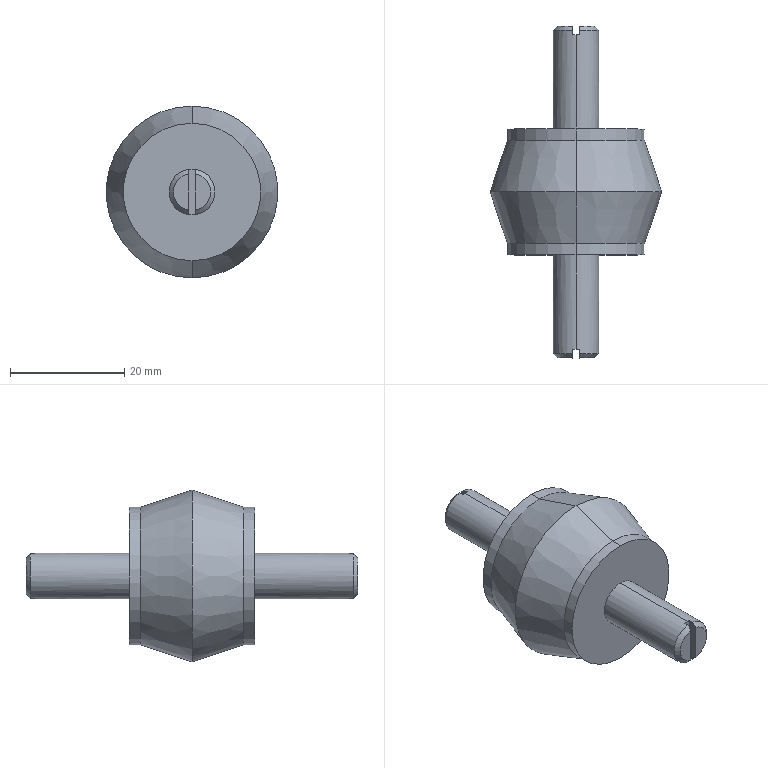Part | SolidWorks | features BaseBody 1 | 1 solid | 28 faces | box 30 x 58 x 30 mm | volume 13926 mm3 | plane 12 | cylinder 8 | cone 8 | commonest cylinder face diameters 8 x4 24 x4
STEP:
#1=CARTESIAN_POINT('',(0.,0.,12.));
#2=VERTEX_POINT('',#1);
#3=CARTESIAN_POINT('',(0.,0.,-12.));
#4=VERTEX_POINT('',#3);
#5=CARTESIAN_POINT('',(0.,0.,0.));
#6=DIRECTION('',(0.,1.,0.));
#7=DIRECTION('',(0.,0.,1.));
#8=AXIS2_PLACEMENT_3D('',#5,#6,#7);
#9=CIRCLE('',#8,12.);
#10=EDGE_CURVE('',#2,#4,#9,.T.);
#11=ORIENTED_EDGE('',*,*,#10,.T.);
#12=CARTESIAN_POINT('',(0.,2.,-12.));
#13=VERTEX_POINT('',#12);
#14=CARTESIAN_POINT('',(0.,0.,-12.));
#15=DIRECTION('',(0.,1.,0.));
#16=VECTOR('',#15,1000.);
#17=LINE('',#14,#16);
#18=EDGE_CURVE('',#4,#13,#17,.T.);
#19=ORIENTED_EDGE('',*,*,#18,.T.);
#20=CARTESIAN_POINT('',(0.,2.,12.));
#21=VERTEX_POINT('',#20);
#22=CARTESIAN_POINT('',(0.,2.,0.));
#23=DIRECTION('',(0.,1.,0.));
#24=DIRECTION('',(0.,0.,1.));
#25=AXIS2_PLACEMENT_3D('',#22,#23,#24);
#26=CIRCLE('',#25,12.);
#27=EDGE_CURVE('',#21,#13,#26,.T.);
#28=ORIENTED_EDGE('',*,*,#27,.F.);
#29=CARTESIAN_POINT('',(0.,0.,12.));
#30=DIRECTION('',(0.,1.,0.));
#31=VECTOR('',#30,1000.);
#32=LINE('',#29,#31);
#33=EDGE_CURVE('',#2,#21,#32,.T.);
#34=ORIENTED_EDGE('',*,*,#33,.F.);
#35=EDGE_LOOP('',(#11,#19,#28,#34));
#36=FACE_OUTER_BOUND('',#35,.T.);
#37=CARTESIAN_POINT('',(0.,0.,0.));
#38=DIRECTION('',(0.,1.,0.));
#39=DIRECTION('',(0.,0.,1.));
#40=AXIS2_PLACEMENT_3D('',#37,#38,#39);
#41=CYLINDRICAL_SURFACE('',#40,12.);
#42=ADVANCED_FACE('',(#36),#41,.T.);
#43=ORIENTED_EDGE('',*,*,#27,.T.);
#44=CARTESIAN_POINT('',(0.,11.,-15.));
#45=VERTEX_POINT('',#44);
#46=CARTESIAN_POINT('',(0.,2.,-12.));
#47=DIRECTION('',(0.,0.9487,-0.3162));
#48=VECTOR('',#47,1000.);
#49=LINE('',#46,#48);
#50=EDGE_CURVE('',#13,#45,#49,.T.);
#51=ORIENTED_EDGE('',*,*,#50,.T.);
#52=CARTESIAN_POINT('',(0.,11.,15.));
#53=VERTEX_POINT('',#52);
#54=CARTESIAN_POINT('',(0.,11.,0.));
#55=DIRECTION('',(0.,1.,0.));
#56=DIRECTION('',(0.,0.,1.));
#57=AXIS2_PLACEMENT_3D('',#54,#55,#56);
#58=CIRCLE('',#57,15.);
#59=EDGE_CURVE('',#53,#45,#58,.T.);
#60=ORIENTED_EDGE('',*,*,#59,.F.);
#61=CARTESIAN_POINT('',(0.,2.,12.));
#62=DIRECTION('',(0.,0.9487,0.3162));
#63=VECTOR('',#62,1000.);
#64=LINE('',#61,#63);
#65=EDGE_CURVE('',#21,#53,#64,.T.);
#66=ORIENTED_EDGE('',*,*,#65,.F.);
#67=EDGE_LOOP('',(#43,#51,#60,#66));
#68=FACE_OUTER_BOUND('',#67,.T.);
#69=CARTESIAN_POINT('',(0.,2.,0.));
#70=DIRECTION('',(0.,1.,0.));
#71=DIRECTION('',(0.,0.,1.));
#72=AXIS2_PLACEMENT_3D('',#69,#70,#71);
#73=CONICAL_SURFACE('',#72,12.,0.3218);
#74=ADVANCED_FACE('',(#68),#73,.T.);
#75=CARTESIAN_POINT('',(0.,20.,12.));
#76=VERTEX_POINT('',#75);
#77=CARTESIAN_POINT('',(0.,20.,-12.));
#78=VERTEX_POINT('',#77);
#79=CARTESIAN_POINT('',(0.,20.,0.));
#80=DIRECTION('',(0.,1.,0.));
#81=DIRECTION('',(0.,0.,1.));
#82=AXIS2_PLACEMENT_3D('',#79,#80,#81);
#83=CIRCLE('',#82,12.);
#84=EDGE_CURVE('',#76,#78,#83,.T.);
#85=ORIENTED_EDGE('',*,*,#84,.F.);
#86=CARTESIAN_POINT('',(0.,11.,15.));
#87=DIRECTION('',(0.,-0.9487,0.3162));
#88=VECTOR('',#87,1000.);
#89=LINE('',#86,#88);
#90=EDGE_CURVE('',#76,#53,#89,.T.);
#91=ORIENTED_EDGE('',*,*,#90,.T.);
#92=ORIENTED_EDGE('',*,*,#59,.T.);
#93=CARTESIAN_POINT('',(0.,11.,-15.));
#94=DIRECTION('',(0.,-0.9487,-0.3162));
#95=VECTOR('',#94,1000.);
#96=LINE('',#93,#95);
#97=EDGE_CURVE('',#78,#45,#96,.T.);
#98=ORIENTED_EDGE('',*,*,#97,.F.);
#99=EDGE_LOOP('',(#85,#91,#92,#98));
#100=FACE_OUTER_BOUND('',#99,.T.);
#101=CARTESIAN_POINT('',(0.,11.,0.));
#102=DIRECTION('',(0.,-1.,0.));
#103=DIRECTION('',(0.,0.,-1.));
#104=AXIS2_PLACEMENT_3D('',#101,#102,#103);
#105=CONICAL_SURFACE('',#104,15.,0.3218);
#106=ADVANCED_FACE('',(#100),#105,.T.);
#107=ORIENTED_EDGE('',*,*,#84,.T.);
#108=CARTESIAN_POINT('',(0.,22.,-12.));
#109=VERTEX_POINT('',#108);
#110=CARTESIAN_POINT('',(0.,0.,-12.));
#111=DIRECTION('',(0.,1.,0.));
#112=VECTOR('',#111,1000.);
#113=LINE('',#110,#112);
#114=EDGE_CURVE('',#78,#109,#113,.T.);
#115=ORIENTED_EDGE('',*,*,#114,.T.);
#116=CARTESIAN_POINT('',(0.,22.,12.));
#117=VERTEX_POINT('',#116);
#118=CARTESIAN_POINT('',(0.,22.,0.));
#119=DIRECTION('',(0.,1.,0.));
#120=DIRECTION('',(0.,0.,1.));
#121=AXIS2_PLACEMENT_3D('',#118,#119,#120);
#122=CIRCLE('',#121,12.);
#123=EDGE_CURVE('',#117,#109,#122,.T.);
#124=ORIENTED_EDGE('',*,*,#123,.F.);
#125=CARTESIAN_POINT('',(0.,0.,12.));
#126=DIRECTION('',(0.,1.,0.));
#127=VECTOR('',#126,1000.);
#128=LINE('',#125,#127);
#129=EDGE_CURVE('',#76,#117,#128,.T.);
#130=ORIENTED_EDGE('',*,*,#129,.F.);
#131=EDGE_LOOP('',(#107,#115,#124,#130));
#132=FACE_OUTER_BOUND('',#131,.T.);
#133=CARTESIAN_POINT('',(0.,0.,0.));
#134=DIRECTION('',(0.,1.,0.));
#135=DIRECTION('',(0.,0.,1.));
#136=AXIS2_PLACEMENT_3D('',#133,#134,#135);
#137=CYLINDRICAL_SURFACE('',#136,12.);
#138=ADVANCED_FACE('',(#132),#137,.T.);
#139=CARTESIAN_POINT('',(0.,22.,4.));
#140=VERTEX_POINT('',#139);
#141=CARTESIAN_POINT('',(0.,22.,-4.));
#142=VERTEX_POINT('',#141);
#143=CARTESIAN_POINT('',(0.,22.,0.));
#144=DIRECTION('',(0.,1.,0.));
#145=DIRECTION('',(0.,0.,-1.));
#146=AXIS2_PLACEMENT_3D('',#143,#144,#145);
#147=CIRCLE('',#146,4.);
#148=EDGE_CURVE('',#140,#142,#147,.T.);
#149=ORIENTED_EDGE('',*,*,#148,.T.);
#150=CARTESIAN_POINT('',(0.,38.5,-4.));
#151=VERTEX_POINT('',#150);
#152=CARTESIAN_POINT('',(0.,22.,-4.));
#153=DIRECTION('',(0.,1.,0.));
#154=VECTOR('',#153,1000.);
#155=LINE('',#152,#154);
#156=EDGE_CURVE('',#142,#151,#155,.T.);
#157=ORIENTED_EDGE('',*,*,#156,.T.);
#158=CARTESIAN_POINT('',(0.6,38.5,-3.955));
#159=VERTEX_POINT('',#158);
#160=CARTESIAN_POINT('',(0.,38.5,0.));
#161=DIRECTION('',(0.,1.,0.));
#162=DIRECTION('',(0.,0.,1.));
#163=AXIS2_PLACEMENT_3D('',#160,#161,#162);
#164=CIRCLE('',#163,4.);
#165=EDGE_CURVE('',#159,#151,#164,.T.);
#166=ORIENTED_EDGE('',*,*,#165,.F.);
#167=CARTESIAN_POINT('',(0.6,39.233,-3.955));
#168=VERTEX_POINT('',#167);
#169=CARTESIAN_POINT('',(0.6,22.,-3.955));
#170=DIRECTION('',(0.,-1.,0.));
#171=VECTOR('',#170,1000.);
#172=LINE('',#169,#171);
#173=EDGE_CURVE('',#168,#159,#172,.T.);
#174=ORIENTED_EDGE('',*,*,#173,.F.);
#175=CARTESIAN_POINT('',(0.6,39.233,3.955));
#176=VERTEX_POINT('',#175);
#177=CARTESIAN_POINT('',(0.,39.233,0.));
#178=DIRECTION('',(0.,1.,0.));
#179=DIRECTION('',(0.,0.,1.));
#180=AXIS2_PLACEMENT_3D('',#177,#178,#179);
#181=CIRCLE('',#180,4.);
#182=EDGE_CURVE('',#176,#168,#181,.T.);
#183=ORIENTED_EDGE('',*,*,#182,.F.);
#184=CARTESIAN_POINT('',(0.6,38.5,3.955));
#185=VERTEX_POINT('',#184);
#186=CARTESIAN_POINT('',(0.6,22.,3.955));
#187=DIRECTION('',(0.,1.,0.));
#188=VECTOR('',#187,1000.);
#189=LINE('',#186,#188);
#190=EDGE_CURVE('',#185,#176,#189,.T.);
#191=ORIENTED_EDGE('',*,*,#190,.F.);
#192=CARTESIAN_POINT('',(0.,38.5,4.));
#193=VERTEX_POINT('',#192);
#194=CARTESIAN_POINT('',(0.,38.5,0.));
#195=DIRECTION('',(0.,1.,0.));
#196=DIRECTION('',(0.,0.,1.));
#197=AXIS2_PLACEMENT_3D('',#194,#195,#196);
#198=CIRCLE('',#197,4.);
#199=EDGE_CURVE('',#193,#185,#198,.T.);
#200=ORIENTED_EDGE('',*,*,#199,.F.);
#201=CARTESIAN_POINT('',(0.,22.,4.));
#202=DIRECTION('',(0.,1.,0.));
#203=VECTOR('',#202,1000.);
#204=LINE('',#201,#203);
#205=EDGE_CURVE('',#140,#193,#204,.T.);
#206=ORIENTED_EDGE('',*,*,#205,.F.);
#207=EDGE_LOOP('',(#149,#157,#166,#174,#183,#191,#200,#206));
#208=FACE_OUTER_BOUND('',#207,.T.);
#209=CARTESIAN_POINT('',(0.,22.,0.));
#210=DIRECTION('',(0.,1.,0.));
#211=DIRECTION('',(0.,0.,1.));
#212=AXIS2_PLACEMENT_3D('',#209,#210,#211);
#213=CYLINDRICAL_SURFACE('',#212,4.);
#214=ADVANCED_FACE('',(#208),#213,.T.);
#215=CARTESIAN_POINT('',(0.,0.,-4.));
#216=VERTEX_POINT('',#215);
#217=CARTESIAN_POINT('',(0.,0.,4.));
#218=VERTEX_POINT('',#217);
#219=CARTESIAN_POINT('',(0.,0.,0.));
#220=DIRECTION('',(0.,-1.,0.));
#221=DIRECTION('',(0.,0.,1.));
#222=AXIS2_PLACEMENT_3D('',#219,#220,#221);
#223=CIRCLE('',#222,4.);
#224=EDGE_CURVE('',#216,#218,#223,.T.);
#225=ORIENTED_EDGE('',*,*,#224,.T.);
#226=CARTESIAN_POINT('',(0.,-16.5,4.));
#227=VERTEX_POINT('',#226);
#228=CARTESIAN_POINT('',(0.,0.,4.));
#229=DIRECTION('',(0.,-1.,0.));
#230=VECTOR('',#229,1000.);
#231=LINE('',#228,#230);
#232=EDGE_CURVE('',#218,#227,#231,.T.);
#233=ORIENTED_EDGE('',*,*,#232,.T.);
#234=CARTESIAN_POINT('',(0.6,-16.5,3.955));
#235=VERTEX_POINT('',#234);
#236=CARTESIAN_POINT('',(0.,-16.5,0.));
#237=DIRECTION('',(0.,-1.,0.));
#238=DIRECTION('',(0.,0.,-1.));
#239=AXIS2_PLACEMENT_3D('',#236,#237,#238);
#240=CIRCLE('',#239,4.);
#241=EDGE_CURVE('',#235,#227,#240,.T.);
#242=ORIENTED_EDGE('',*,*,#241,.F.);
#243=CARTESIAN_POINT('',(0.6,-17.233,3.955));
#244=VERTEX_POINT('',#243);
#245=CARTESIAN_POINT('',(0.6,0.,3.955));
#246=DIRECTION('',(0.,1.,0.));
#247=VECTOR('',#246,1000.);
#248=LINE('',#245,#247);
#249=EDGE_CURVE('',#244,#235,#248,.T.);
#250=ORIENTED_EDGE('',*,*,#249,.F.);
#251=CARTESIAN_POINT('',(0.6,-17.233,-3.955));
#252=VERTEX_POINT('',#251);
#253=CARTESIAN_POINT('',(0.,-17.233,0.));
#254=DIRECTION('',(0.,-1.,0.));
#255=DIRECTION('',(0.,0.,-1.));
#256=AXIS2_PLACEMENT_3D('',#253,#254,#255);
#257=CIRCLE('',#256,4.);
#258=EDGE_CURVE('',#252,#244,#257,.T.);
#259=ORIENTED_EDGE('',*,*,#258,.F.);
#260=CARTESIAN_POINT('',(0.6,-16.5,-3.955));
#261=VERTEX_POINT('',#260);
#262=CARTESIAN_POINT('',(0.6,0.,-3.955));
#263=DIRECTION('',(0.,-1.,0.));
#264=VECTOR('',#263,1000.);
#265=LINE('',#262,#264);
#266=EDGE_CURVE('',#261,#252,#265,.T.);
#267=ORIENTED_EDGE('',*,*,#266,.F.);
#268=CARTESIAN_POINT('',(0.,-16.5,-4.));
#269=VERTEX_POINT('',#268);
#270=CARTESIAN_POINT('',(0.,-16.5,0.));
#271=DIRECTION('',(0.,-1.,0.));
#272=DIRECTION('',(0.,0.,-1.));
#273=AXIS2_PLACEMENT_3D('',#270,#271,#272);
#274=CIRCLE('',#273,4.);
#275=EDGE_CURVE('',#269,#261,#274,.T.);
#276=ORIENTED_EDGE('',*,*,#275,.F.);
#277=CARTESIAN_POINT('',(0.,0.,-4.));
#278=DIRECTION('',(0.,-1.,0.));
#279=VECTOR('',#278,1000.);
#280=LINE('',#277,#279);
#281=EDGE_CURVE('',#216,#269,#280,.T.);
#282=ORIENTED_EDGE('',*,*,#281,.F.);
#283=EDGE_LOOP('',(#225,#233,#242,#250,#259,#267,#276,#282));
#284=FACE_OUTER_BOUND('',#283,.T.);
#285=CARTESIAN_POINT('',(0.,0.,0.));
#286=DIRECTION('',(0.,-1.,0.));
#287=DIRECTION('',(0.,0.,-1.));
#288=AXIS2_PLACEMENT_3D('',#285,#286,#287);
#289=CYLINDRICAL_SURFACE('',#288,4.);
#290=ADVANCED_FACE('',(#284),#289,.T.);
#291=CARTESIAN_POINT('',(0.6,-16.5,4.));
#292=DIRECTION('',(0.,0.,-1.));
#293=VECTOR('',#292,1000.);
#294=LINE('',#291,#293);
#295=EDGE_CURVE('',#235,#261,#294,.T.);
#296=ORIENTED_EDGE('',*,*,#295,.F.);
#297=ORIENTED_EDGE('',*,*,#241,.T.);
#298=CARTESIAN_POINT('',(-0.6,-16.5,3.955));
#299=VERTEX_POINT('',#298);
#300=CARTESIAN_POINT('',(0.,-16.5,0.));
#301=DIRECTION('',(0.,-1.,0.));
#302=DIRECTION('',(0.,0.,-1.));
#303=AXIS2_PLACEMENT_3D('',#300,#301,#302);
#304=CIRCLE('',#303,4.);
#305=EDGE_CURVE('',#227,#299,#304,.T.);
#306=ORIENTED_EDGE('',*,*,#305,.T.);
#307=CARTESIAN_POINT('',(-0.6,-16.5,-3.955));
#308=VERTEX_POINT('',#307);
#309=CARTESIAN_POINT('',(-0.6,-16.5,4.));
#310=DIRECTION('',(0.,0.,-1.));
#311=VECTOR('',#310,1000.);
#312=LINE('',#309,#311);
#313=EDGE_CURVE('',#299,#308,#312,.T.);
#314=ORIENTED_EDGE('',*,*,#313,.T.);
#315=CARTESIAN_POINT('',(0.,-16.5,0.));
#316=DIRECTION('',(0.,-1.,0.));
#317=DIRECTION('',(0.,0.,-1.));
#318=AXIS2_PLACEMENT_3D('',#315,#316,#317);
#319=CIRCLE('',#318,4.);
#320=EDGE_CURVE('',#308,#269,#319,.T.);
#321=ORIENTED_EDGE('',*,*,#320,.T.);
#322=ORIENTED_EDGE('',*,*,#275,.T.);
#323=EDGE_LOOP('',(#296,#297,#306,#314,#321,#322));
#324=FACE_OUTER_BOUND('',#323,.T.);
#325=CARTESIAN_POINT('',(0.6,-16.5,4.));
#326=DIRECTION('',(0.,-1.,0.));
#327=DIRECTION('',(0.,0.,-1.));
#328=AXIS2_PLACEMENT_3D('',#325,#326,#327);
#329=PLANE('',#328);
#330=ADVANCED_FACE('',(#324),#329,.T.);
#331=CARTESIAN_POINT('',(0.6,-18.,-3.177));
#332=VERTEX_POINT('',#331);
#333=CARTESIAN_POINT('',(0.6,-17.233,-3.955));
#334=CARTESIAN_POINT('',(0.6,-17.489,-3.696));
#335=CARTESIAN_POINT('',(0.6,-17.745,-3.437));
#336=CARTESIAN_POINT('',(0.6,-18.,-3.177));
#337=B_SPLINE_CURVE_WITH_KNOTS('',3,(#333,#334,#335,#336),.UNSPECIFIED.,.F.,.F.,(4,4),(0.006837,0.00793),.UNSPECIFIED.);
#338=EDGE_CURVE('',#252,#332,#337,.T.);
#339=ORIENTED_EDGE('',*,*,#338,.T.);
#340=CARTESIAN_POINT('',(0.6,-18.,3.177));
#341=VERTEX_POINT('',#340);
#342=CARTESIAN_POINT('',(0.6,-18.,4.));
#343=DIRECTION('',(0.,0.,-1.));
#344=VECTOR('',#343,1000.);
#345=LINE('',#342,#344);
#346=EDGE_CURVE('',#341,#332,#345,.T.);
#347=ORIENTED_EDGE('',*,*,#346,.F.);
#348=CARTESIAN_POINT('',(0.6,-18.,3.177));
#349=CARTESIAN_POINT('',(0.6,-17.745,3.437));
#350=CARTESIAN_POINT('',(0.6,-17.489,3.696));
#351=CARTESIAN_POINT('',(0.6,-17.233,3.955));
#352=B_SPLINE_CURVE_WITH_KNOTS('',3,(#348,#349,#350,#351),.UNSPECIFIED.,.F.,.F.,(4,4),(0.01631,0.01741),.UNSPECIFIED.);
#353=EDGE_CURVE('',#341,#244,#352,.T.);
#354=ORIENTED_EDGE('',*,*,#353,.T.);
#355=ORIENTED_EDGE('',*,*,#249,.T.);
#356=ORIENTED_EDGE('',*,*,#295,.T.);
#357=ORIENTED_EDGE('',*,*,#266,.T.);
#358=EDGE_LOOP('',(#339,#347,#354,#355,#356,#357));
#359=FACE_OUTER_BOUND('',#358,.T.);
#360=CARTESIAN_POINT('',(0.6,-18.,4.));
#361=DIRECTION('',(-1.,0.,0.));
#362=DIRECTION('',(0.,0.,1.));
#363=AXIS2_PLACEMENT_3D('',#360,#361,#362);
#364=PLANE('',#363);
#365=ADVANCED_FACE('',(#359),#364,.T.);
#366=CARTESIAN_POINT('',(-0.6,-17.233,3.955));
#367=VERTEX_POINT('',#366);
#368=CARTESIAN_POINT('',(-0.6,-18.,3.177));
#369=VERTEX_POINT('',#368);
#370=CARTESIAN_POINT('',(-0.6,-17.233,3.955));
#371=CARTESIAN_POINT('',(-0.6,-17.489,3.696));
#372=CARTESIAN_POINT('',(-0.6,-17.745,3.437));
#373=CARTESIAN_POINT('',(-0.6,-18.,3.177));
#374=B_SPLINE_CURVE_WITH_KNOTS('',3,(#370,#371,#372,#373),.UNSPECIFIED.,.F.,.F.,(4,4),(0.006837,0.00793),.UNSPECIFIED.);
#375=EDGE_CURVE('',#367,#369,#374,.T.);
#376=ORIENTED_EDGE('',*,*,#375,.T.);
#377=CARTESIAN_POINT('',(-0.6,-18.,-3.177));
#378=VERTEX_POINT('',#377);
#379=CARTESIAN_POINT('',(-0.6,-18.,4.));
#380=DIRECTION('',(0.,0.,-1.));
#381=VECTOR('',#380,1000.);
#382=LINE('',#379,#381);
#383=EDGE_CURVE('',#369,#378,#382,.T.);
#384=ORIENTED_EDGE('',*,*,#383,.T.);
#385=CARTESIAN_POINT('',(-0.6,-17.233,-3.955));
#386=VERTEX_POINT('',#385);
#387=CARTESIAN_POINT('',(-0.6,-18.,-3.177));
#388=CARTESIAN_POINT('',(-0.6,-17.745,-3.437));
#389=CARTESIAN_POINT('',(-0.6,-17.489,-3.696));
#390=CARTESIAN_POINT('',(-0.6,-17.233,-3.955));
#391=B_SPLINE_CURVE_WITH_KNOTS('',3,(#387,#388,#389,#390),.UNSPECIFIED.,.F.,.F.,(4,4),(0.01631,0.01741),.UNSPECIFIED.);
#392=EDGE_CURVE('',#378,#386,#391,.T.);
#393=ORIENTED_EDGE('',*,*,#392,.T.);
#394=CARTESIAN_POINT('',(-0.6,0.,-3.955));
#395=DIRECTION('',(0.,1.,0.));
#396=VECTOR('',#395,1000.);
#397=LINE('',#394,#396);
#398=EDGE_CURVE('',#386,#308,#397,.T.);
#399=ORIENTED_EDGE('',*,*,#398,.T.);
#400=ORIENTED_EDGE('',*,*,#313,.F.);
#401=CARTESIAN_POINT('',(-0.6,0.,3.955));
#402=DIRECTION('',(0.,-1.,0.));
#403=VECTOR('',#402,1000.);
#404=LINE('',#401,#403);
#405=EDGE_CURVE('',#299,#367,#404,.T.);
#406=ORIENTED_EDGE('',*,*,#405,.T.);
#407=EDGE_LOOP('',(#376,#384,#393,#399,#400,#406));
#408=FACE_OUTER_BOUND('',#407,.T.);
#409=CARTESIAN_POINT('',(-0.6,-16.5,4.));
#410=DIRECTION('',(1.,0.,0.));
#411=DIRECTION('',(0.,1.,0.));
#412=AXIS2_PLACEMENT_3D('',#409,#410,#411);
#413=PLANE('',#412);
#414=ADVANCED_FACE('',(#408),#413,.T.);
#415=CARTESIAN_POINT('',(0.6,40.,3.177));
#416=VERTEX_POINT('',#415);
#417=CARTESIAN_POINT('',(0.6,39.233,3.955));
#418=CARTESIAN_POINT('',(0.6,39.489,3.696));
#419=CARTESIAN_POINT('',(0.6,39.745,3.437));
#420=CARTESIAN_POINT('',(0.6,40.,3.177));
#421=B_SPLINE_CURVE_WITH_KNOTS('',3,(#417,#418,#419,#420),.UNSPECIFIED.,.F.,.F.,(4,4),(0.006837,0.00793),.UNSPECIFIED.);
#422=EDGE_CURVE('',#176,#416,#421,.T.);
#423=ORIENTED_EDGE('',*,*,#422,.T.);
#424=CARTESIAN_POINT('',(0.6,40.,-3.177));
#425=VERTEX_POINT('',#424);
#426=CARTESIAN_POINT('',(0.6,40.,4.));
#427=DIRECTION('',(0.,0.,-1.));
#428=VECTOR('',#427,1000.);
#429=LINE('',#426,#428);
#430=EDGE_CURVE('',#416,#425,#429,.T.);
#431=ORIENTED_EDGE('',*,*,#430,.T.);
#432=CARTESIAN_POINT('',(0.6,40.,-3.177));
#433=CARTESIAN_POINT('',(0.6,39.745,-3.437));
#434=CARTESIAN_POINT('',(0.6,39.489,-3.696));
#435=CARTESIAN_POINT('',(0.6,39.233,-3.955));
#436=B_SPLINE_CURVE_WITH_KNOTS('',3,(#432,#433,#434,#435),.UNSPECIFIED.,.F.,.F.,(4,4),(0.01631,0.01741),.UNSPECIFIED.);
#437=EDGE_CURVE('',#425,#168,#436,.T.);
#438=ORIENTED_EDGE('',*,*,#437,.T.);
#439=ORIENTED_EDGE('',*,*,#173,.T.);
#440=CARTESIAN_POINT('',(0.6,38.5,4.));
#441=DIRECTION('',(0.,0.,-1.));
#442=VECTOR('',#441,1000.);
#443=LINE('',#440,#442);
#444=EDGE_CURVE('',#185,#159,#443,.T.);
#445=ORIENTED_EDGE('',*,*,#444,.F.);
#446=ORIENTED_EDGE('',*,*,#190,.T.);
#447=EDGE_LOOP('',(#423,#431,#438,#439,#445,#446));
#448=FACE_OUTER_BOUND('',#447,.T.);
#449=CARTESIAN_POINT('',(0.6,38.5,4.));
#450=DIRECTION('',(-1.,0.,0.));
#451=DIRECTION('',(0.,0.,1.));
#452=AXIS2_PLACEMENT_3D('',#449,#450,#451);
#453=PLANE('',#452);
#454=ADVANCED_FACE('',(#448),#453,.T.);
#455=ORIENTED_EDGE('',*,*,#444,.T.);
#456=ORIENTED_EDGE('',*,*,#165,.T.);
#457=CARTESIAN_POINT('',(-0.6,38.5,-3.955));
#458=VERTEX_POINT('',#457);
#459=CARTESIAN_POINT('',(0.,38.5,0.));
#460=DIRECTION('',(0.,1.,0.));
#461=DIRECTION('',(0.,0.,1.));
#462=AXIS2_PLACEMENT_3D('',#459,#460,#461);
#463=CIRCLE('',#462,4.);
#464=EDGE_CURVE('',#151,#458,#463,.T.);
#465=ORIENTED_EDGE('',*,*,#464,.T.);
#466=CARTESIAN_POINT('',(-0.6,38.5,3.955));
#467=VERTEX_POINT('',#466);
#468=CARTESIAN_POINT('',(-0.6,38.5,4.));
#469=DIRECTION('',(0.,0.,-1.));
#470=VECTOR('',#469,1000.);
#471=LINE('',#468,#470);
#472=EDGE_CURVE('',#467,#458,#471,.T.);
#473=ORIENTED_EDGE('',*,*,#472,.F.);
#474=CARTESIAN_POINT('',(0.,38.5,0.));
#475=DIRECTION('',(0.,1.,0.));
#476=DIRECTION('',(0.,0.,1.));
#477=AXIS2_PLACEMENT_3D('',#474,#475,#476);
#478=CIRCLE('',#477,4.);
#479=EDGE_CURVE('',#467,#193,#478,.T.);
#480=ORIENTED_EDGE('',*,*,#479,.T.);
#481=ORIENTED_EDGE('',*,*,#199,.T.);
#482=EDGE_LOOP('',(#455,#456,#465,#473,#480,#481));
#483=FACE_OUTER_BOUND('',#482,.T.);
#484=CARTESIAN_POINT('',(-0.6,38.5,4.));
#485=DIRECTION('',(0.,1.,0.));
#486=DIRECTION('',(1.,0.,0.));
#487=AXIS2_PLACEMENT_3D('',#484,#485,#486);
#488=PLANE('',#487);
#489=ADVANCED_FACE('',(#483),#488,.T.);
#490=CARTESIAN_POINT('',(-0.6,39.233,-3.955));
#491=VERTEX_POINT('',#490);
#492=CARTESIAN_POINT('',(-0.6,40.,-3.177));
#493=VERTEX_POINT('',#492);
#494=CARTESIAN_POINT('',(-0.6,39.233,-3.955));
#495=CARTESIAN_POINT('',(-0.6,39.489,-3.696));
#496=CARTESIAN_POINT('',(-0.6,39.745,-3.437));
#497=CARTESIAN_POINT('',(-0.6,40.,-3.177));
#498=B_SPLINE_CURVE_WITH_KNOTS('',3,(#494,#495,#496,#497),.UNSPECIFIED.,.F.,.F.,(4,4),(0.006837,0.00793),.UNSPECIFIED.);
#499=EDGE_CURVE('',#491,#493,#498,.T.);
#500=ORIENTED_EDGE('',*,*,#499,.T.);
#501=CARTESIAN_POINT('',(-0.6,40.,3.177));
#502=VERTEX_POINT('',#501);
#503=CARTESIAN_POINT('',(-0.6,40.,4.));
#504=DIRECTION('',(0.,0.,-1.));
#505=VECTOR('',#504,1000.);
#506=LINE('',#503,#505);
#507=EDGE_CURVE('',#502,#493,#506,.T.);
#508=ORIENTED_EDGE('',*,*,#507,.F.);
#509=CARTESIAN_POINT('',(-0.6,39.233,3.955));
#510=VERTEX_POINT('',#509);
#511=CARTESIAN_POINT('',(-0.6,40.,3.177));
#512=CARTESIAN_POINT('',(-0.6,39.745,3.437));
#513=CARTESIAN_POINT('',(-0.6,39.489,3.696));
#514=CARTESIAN_POINT('',(-0.6,39.233,3.955));
#515=B_SPLINE_CURVE_WITH_KNOTS('',3,(#511,#512,#513,#514),.UNSPECIFIED.,.F.,.F.,(4,4),(0.01631,0.01741),.UNSPECIFIED.);
#516=EDGE_CURVE('',#502,#510,#515,.T.);
#517=ORIENTED_EDGE('',*,*,#516,.T.);
#518=CARTESIAN_POINT('',(-0.6,22.,3.955));
#519=DIRECTION('',(0.,-1.,0.));
#520=VECTOR('',#519,1000.);
#521=LINE('',#518,#520);
#522=EDGE_CURVE('',#510,#467,#521,.T.);
#523=ORIENTED_EDGE('',*,*,#522,.T.);
#524=ORIENTED_EDGE('',*,*,#472,.T.);
#525=CARTESIAN_POINT('',(-0.6,22.,-3.955));
#526=DIRECTION('',(0.,1.,0.));
#527=VECTOR('',#526,1000.);
#528=LINE('',#525,#527);
#529=EDGE_CURVE('',#458,#491,#528,.T.);
#530=ORIENTED_EDGE('',*,*,#529,.T.);
#531=EDGE_LOOP('',(#500,#508,#517,#523,#524,#530));
#532=FACE_OUTER_BOUND('',#531,.T.);
#533=CARTESIAN_POINT('',(-0.6,40.,4.));
#534=DIRECTION('',(1.,0.,0.));
#535=DIRECTION('',(0.,1.,0.));
#536=AXIS2_PLACEMENT_3D('',#533,#534,#535);
#537=PLANE('',#536);
#538=ADVANCED_FACE('',(#532),#537,.T.);
#539=ORIENTED_EDGE('',*,*,#224,.F.);
#540=CARTESIAN_POINT('',(0.,0.,0.));
#541=DIRECTION('',(0.,-1.,0.));
#542=DIRECTION('',(0.,0.,1.));
#543=AXIS2_PLACEMENT_3D('',#540,#541,#542);
#544=CIRCLE('',#543,4.);
#545=EDGE_CURVE('',#218,#216,#544,.T.);
#546=ORIENTED_EDGE('',*,*,#545,.F.);
#547=EDGE_LOOP('',(#539,#546));
#548=FACE_BOUND('',#547,.T.);
#549=ORIENTED_EDGE('',*,*,#10,.F.);
#550=CARTESIAN_POINT('',(0.,0.,0.));
#551=DIRECTION('',(0.,1.,0.));
#552=DIRECTION('',(0.,0.,1.));
#553=AXIS2_PLACEMENT_3D('',#550,#551,#552);
#554=CIRCLE('',#553,12.);
#555=EDGE_CURVE('',#4,#2,#554,.T.);
#556=ORIENTED_EDGE('',*,*,#555,.F.);
#557=EDGE_LOOP('',(#549,#556));
#558=FACE_OUTER_BOUND('',#557,.T.);
#559=CARTESIAN_POINT('',(12.,0.,0.));
#560=DIRECTION('',(0.,1.,0.));
#561=DIRECTION('',(1.,0.,0.));
#562=AXIS2_PLACEMENT_3D('',#559,#560,#561);
#563=PLANE('',#562);
#564=ADVANCED_FACE('',(#548,#558),#563,.F.);
#565=ORIENTED_EDGE('',*,*,#148,.F.);
#566=CARTESIAN_POINT('',(0.,22.,0.));
#567=DIRECTION('',(0.,1.,0.));
#568=DIRECTION('',(0.,0.,-1.));
#569=AXIS2_PLACEMENT_3D('',#566,#567,#568);
#570=CIRCLE('',#569,4.);
#571=EDGE_CURVE('',#142,#140,#570,.T.);
#572=ORIENTED_EDGE('',*,*,#571,.F.);
#573=EDGE_LOOP('',(#565,#572));
#574=FACE_BOUND('',#573,.T.);
#575=ORIENTED_EDGE('',*,*,#123,.T.);
#576=CARTESIAN_POINT('',(0.,22.,0.));
#577=DIRECTION('',(0.,1.,0.));
#578=DIRECTION('',(0.,0.,1.));
#579=AXIS2_PLACEMENT_3D('',#576,#577,#578);
#580=CIRCLE('',#579,12.);
#581=EDGE_CURVE('',#109,#117,#580,.T.);
#582=ORIENTED_EDGE('',*,*,#581,.T.);
#583=EDGE_LOOP('',(#575,#582));
#584=FACE_OUTER_BOUND('',#583,.T.);
#585=CARTESIAN_POINT('',(0.,22.,0.));
#586=DIRECTION('',(0.,-1.,0.));
#587=DIRECTION('',(0.,0.,-1.));
#588=AXIS2_PLACEMENT_3D('',#585,#586,#587);
#589=PLANE('',#588);
#590=ADVANCED_FACE('',(#574,#584),#589,.F.);
#591=ORIENTED_EDGE('',*,*,#422,.F.);
#592=ORIENTED_EDGE('',*,*,#182,.T.);
#593=ORIENTED_EDGE('',*,*,#437,.F.);
#594=CARTESIAN_POINT('',(0.,40.,0.));
#595=DIRECTION('',(0.,1.,0.));
#596=DIRECTION('',(0.,0.,1.));
#597=AXIS2_PLACEMENT_3D('',#594,#595,#596);
#598=CIRCLE('',#597,3.233);
#599=EDGE_CURVE('',#416,#425,#598,.T.);
#600=ORIENTED_EDGE('',*,*,#599,.F.);
#601=EDGE_LOOP('',(#591,#592,#593,#600));
#602=FACE_OUTER_BOUND('',#601,.T.);
#603=CARTESIAN_POINT('',(0.,39.233,0.));
#604=DIRECTION('',(0.,-1.,0.));
#605=DIRECTION('',(0.,0.,-1.));
#606=AXIS2_PLACEMENT_3D('',#603,#604,#605);
#607=CONICAL_SURFACE('',#606,4.,0.7854);
#608=ADVANCED_FACE('',(#602),#607,.T.);
#609=ORIENTED_EDGE('',*,*,#499,.F.);
#610=CARTESIAN_POINT('',(0.,39.233,0.));
#611=DIRECTION('',(0.,1.,0.));
#612=DIRECTION('',(0.,0.,1.));
#613=AXIS2_PLACEMENT_3D('',#610,#611,#612);
#614=CIRCLE('',#613,4.);
#615=EDGE_CURVE('',#491,#510,#614,.T.);
#616=ORIENTED_EDGE('',*,*,#615,.T.);
#617=ORIENTED_EDGE('',*,*,#516,.F.);
#618=CARTESIAN_POINT('',(0.,40.,0.));
#619=DIRECTION('',(0.,1.,0.));
#620=DIRECTION('',(0.,0.,1.));
#621=AXIS2_PLACEMENT_3D('',#618,#619,#620);
#622=CIRCLE('',#621,3.233);
#623=EDGE_CURVE('',#493,#502,#622,.T.);
#624=ORIENTED_EDGE('',*,*,#623,.F.);
#625=EDGE_LOOP('',(#609,#616,#617,#624));
#626=FACE_OUTER_BOUND('',#625,.T.);
#627=CARTESIAN_POINT('',(0.,39.233,0.));
#628=DIRECTION('',(0.,-1.,0.));
#629=DIRECTION('',(0.,0.,-1.));
#630=AXIS2_PLACEMENT_3D('',#627,#628,#629);
#631=CONICAL_SURFACE('',#630,4.,0.7854);
#632=ADVANCED_FACE('',(#626),#631,.T.);
#633=ORIENTED_EDGE('',*,*,#430,.F.);
#634=ORIENTED_EDGE('',*,*,#599,.T.);
#635=EDGE_LOOP('',(#633,#634));
#636=FACE_OUTER_BOUND('',#635,.T.);
#637=CARTESIAN_POINT('',(0.,40.,0.));
#638=DIRECTION('',(0.,-1.,0.));
#639=DIRECTION('',(0.,0.,-1.));
#640=AXIS2_PLACEMENT_3D('',#637,#638,#639);
#641=PLANE('',#640);
#642=ADVANCED_FACE('',(#636),#641,.F.);
#643=ORIENTED_EDGE('',*,*,#507,.T.);
#644=ORIENTED_EDGE('',*,*,#623,.T.);
#645=EDGE_LOOP('',(#643,#644));
#646=FACE_OUTER_BOUND('',#645,.T.);
#647=CARTESIAN_POINT('',(0.,40.,0.));
#648=DIRECTION('',(0.,-1.,0.));
#649=DIRECTION('',(0.,0.,-1.));
#650=AXIS2_PLACEMENT_3D('',#647,#648,#649);
#651=PLANE('',#650);
#652=ADVANCED_FACE('',(#646),#651,.F.);
#653=ORIENTED_EDGE('',*,*,#338,.F.);
#654=ORIENTED_EDGE('',*,*,#258,.T.);
#655=ORIENTED_EDGE('',*,*,#353,.F.);
#656=CARTESIAN_POINT('',(0.,-18.,0.));
#657=DIRECTION('',(0.,-1.,0.));
#658=DIRECTION('',(0.,0.,-1.));
#659=AXIS2_PLACEMENT_3D('',#656,#657,#658);
#660=CIRCLE('',#659,3.233);
#661=EDGE_CURVE('',#332,#341,#660,.T.);
#662=ORIENTED_EDGE('',*,*,#661,.F.);
#663=EDGE_LOOP('',(#653,#654,#655,#662));
#664=FACE_OUTER_BOUND('',#663,.T.);
#665=CARTESIAN_POINT('',(0.,-17.233,0.));
#666=DIRECTION('',(0.,1.,0.));
#667=DIRECTION('',(0.,0.,1.));
#668=AXIS2_PLACEMENT_3D('',#665,#666,#667);
#669=CONICAL_SURFACE('',#668,4.,0.7854);
#670=ADVANCED_FACE('',(#664),#669,.T.);
#671=ORIENTED_EDGE('',*,*,#375,.F.);
#672=CARTESIAN_POINT('',(0.,-17.233,0.));
#673=DIRECTION('',(0.,-1.,0.));
#674=DIRECTION('',(0.,0.,-1.));
#675=AXIS2_PLACEMENT_3D('',#672,#673,#674);
#676=CIRCLE('',#675,4.);
#677=EDGE_CURVE('',#367,#386,#676,.T.);
#678=ORIENTED_EDGE('',*,*,#677,.T.);
#679=ORIENTED_EDGE('',*,*,#392,.F.);
#680=CARTESIAN_POINT('',(0.,-18.,0.));
#681=DIRECTION('',(0.,-1.,0.));
#682=DIRECTION('',(0.,0.,-1.));
#683=AXIS2_PLACEMENT_3D('',#680,#681,#682);
#684=CIRCLE('',#683,3.233);
#685=EDGE_CURVE('',#369,#378,#684,.T.);
#686=ORIENTED_EDGE('',*,*,#685,.F.);
#687=EDGE_LOOP('',(#671,#678,#679,#686));
#688=FACE_OUTER_BOUND('',#687,.T.);
#689=CARTESIAN_POINT('',(0.,-17.233,0.));
#690=DIRECTION('',(0.,1.,0.));
#691=DIRECTION('',(0.,0.,1.));
#692=AXIS2_PLACEMENT_3D('',#689,#690,#691);
#693=CONICAL_SURFACE('',#692,4.,0.7854);
#694=ADVANCED_FACE('',(#688),#693,.T.);
#695=ORIENTED_EDGE('',*,*,#346,.T.);
#696=ORIENTED_EDGE('',*,*,#661,.T.);
#697=EDGE_LOOP('',(#695,#696));
#698=FACE_OUTER_BOUND('',#697,.T.);
#699=CARTESIAN_POINT('',(0.,-18.,0.));
#700=DIRECTION('',(0.,1.,0.));
#701=DIRECTION('',(1.,0.,0.));
#702=AXIS2_PLACEMENT_3D('',#699,#700,#701);
#703=PLANE('',#702);
#704=ADVANCED_FACE('',(#698),#703,.F.);
#705=ORIENTED_EDGE('',*,*,#383,.F.);
#706=ORIENTED_EDGE('',*,*,#685,.T.);
#707=EDGE_LOOP('',(#705,#706));
#708=FACE_OUTER_BOUND('',#707,.T.);
#709=CARTESIAN_POINT('',(0.,-18.,0.));
#710=DIRECTION('',(0.,1.,0.));
#711=DIRECTION('',(1.,0.,0.));
#712=AXIS2_PLACEMENT_3D('',#709,#710,#711);
#713=PLANE('',#712);
#714=ADVANCED_FACE('',(#708),#713,.F.);
#715=ORIENTED_EDGE('',*,*,#232,.F.);
#716=ORIENTED_EDGE('',*,*,#545,.T.);
#717=ORIENTED_EDGE('',*,*,#281,.T.);
#718=ORIENTED_EDGE('',*,*,#320,.F.);
#719=ORIENTED_EDGE('',*,*,#398,.F.);
#720=ORIENTED_EDGE('',*,*,#677,.F.);
#721=ORIENTED_EDGE('',*,*,#405,.F.);
#722=ORIENTED_EDGE('',*,*,#305,.F.);
#723=EDGE_LOOP('',(#715,#716,#717,#718,#719,#720,#721,#722));
#724=FACE_OUTER_BOUND('',#723,.T.);
#725=CARTESIAN_POINT('',(0.,0.,0.));
#726=DIRECTION('',(0.,-1.,0.));
#727=DIRECTION('',(0.,0.,-1.));
#728=AXIS2_PLACEMENT_3D('',#725,#726,#727);
#729=CYLINDRICAL_SURFACE('',#728,4.);
#730=ADVANCED_FACE('',(#724),#729,.T.);
#731=ORIENTED_EDGE('',*,*,#156,.F.);
#732=ORIENTED_EDGE('',*,*,#571,.T.);
#733=ORIENTED_EDGE('',*,*,#205,.T.);
#734=ORIENTED_EDGE('',*,*,#479,.F.);
#735=ORIENTED_EDGE('',*,*,#522,.F.);
#736=ORIENTED_EDGE('',*,*,#615,.F.);
#737=ORIENTED_EDGE('',*,*,#529,.F.);
#738=ORIENTED_EDGE('',*,*,#464,.F.);
#739=EDGE_LOOP('',(#731,#732,#733,#734,#735,#736,#737,#738));
#740=FACE_OUTER_BOUND('',#739,.T.);
#741=CARTESIAN_POINT('',(0.,22.,0.));
#742=DIRECTION('',(0.,1.,0.));
#743=DIRECTION('',(0.,0.,1.));
#744=AXIS2_PLACEMENT_3D('',#741,#742,#743);
#745=CYLINDRICAL_SURFACE('',#744,4.);
#746=ADVANCED_FACE('',(#740),#745,.T.);
#747=ORIENTED_EDGE('',*,*,#114,.F.);
#748=CARTESIAN_POINT('',(0.,20.,0.));
#749=DIRECTION('',(0.,1.,0.));
#750=DIRECTION('',(0.,0.,1.));
#751=AXIS2_PLACEMENT_3D('',#748,#749,#750);
#752=CIRCLE('',#751,12.);
#753=EDGE_CURVE('',#78,#76,#752,.T.);
#754=ORIENTED_EDGE('',*,*,#753,.T.);
#755=ORIENTED_EDGE('',*,*,#129,.T.);
#756=ORIENTED_EDGE('',*,*,#581,.F.);
#757=EDGE_LOOP('',(#747,#754,#755,#756));
#758=FACE_OUTER_BOUND('',#757,.T.);
#759=CARTESIAN_POINT('',(0.,0.,0.));
#760=DIRECTION('',(0.,1.,0.));
#761=DIRECTION('',(0.,0.,1.));
#762=AXIS2_PLACEMENT_3D('',#759,#760,#761);
#763=CYLINDRICAL_SURFACE('',#762,12.);
#764=ADVANCED_FACE('',(#758),#763,.T.);
#765=ORIENTED_EDGE('',*,*,#90,.F.);
#766=ORIENTED_EDGE('',*,*,#753,.F.);
#767=ORIENTED_EDGE('',*,*,#97,.T.);
#768=CARTESIAN_POINT('',(0.,11.,0.));
#769=DIRECTION('',(0.,1.,0.));
#770=DIRECTION('',(0.,0.,1.));
#771=AXIS2_PLACEMENT_3D('',#768,#769,#770);
#772=CIRCLE('',#771,15.);
#773=EDGE_CURVE('',#45,#53,#772,.T.);
#774=ORIENTED_EDGE('',*,*,#773,.T.);
#775=EDGE_LOOP('',(#765,#766,#767,#774));
#776=FACE_OUTER_BOUND('',#775,.T.);
#777=CARTESIAN_POINT('',(0.,11.,0.));
#778=DIRECTION('',(0.,-1.,0.));
#779=DIRECTION('',(0.,0.,-1.));
#780=AXIS2_PLACEMENT_3D('',#777,#778,#779);
#781=CONICAL_SURFACE('',#780,15.,0.3218);
#782=ADVANCED_FACE('',(#776),#781,.T.);
#783=ORIENTED_EDGE('',*,*,#50,.F.);
#784=CARTESIAN_POINT('',(0.,2.,0.));
#785=DIRECTION('',(0.,1.,0.));
#786=DIRECTION('',(0.,0.,1.));
#787=AXIS2_PLACEMENT_3D('',#784,#785,#786);
#788=CIRCLE('',#787,12.);
#789=EDGE_CURVE('',#13,#21,#788,.T.);
#790=ORIENTED_EDGE('',*,*,#789,.T.);
#791=ORIENTED_EDGE('',*,*,#65,.T.);
#792=ORIENTED_EDGE('',*,*,#773,.F.);
#793=EDGE_LOOP('',(#783,#790,#791,#792));
#794=FACE_OUTER_BOUND('',#793,.T.);
#795=CARTESIAN_POINT('',(0.,2.,0.));
#796=DIRECTION('',(0.,1.,0.));
#797=DIRECTION('',(0.,0.,1.));
#798=AXIS2_PLACEMENT_3D('',#795,#796,#797);
#799=CONICAL_SURFACE('',#798,12.,0.3218);
#800=ADVANCED_FACE('',(#794),#799,.T.);
#801=ORIENTED_EDGE('',*,*,#18,.F.);
#802=ORIENTED_EDGE('',*,*,#555,.T.);
#803=ORIENTED_EDGE('',*,*,#33,.T.);
#804=ORIENTED_EDGE('',*,*,#789,.F.);
#805=EDGE_LOOP('',(#801,#802,#803,#804));
#806=FACE_OUTER_BOUND('',#805,.T.);
#807=CARTESIAN_POINT('',(0.,0.,0.));
#808=DIRECTION('',(0.,1.,0.));
#809=DIRECTION('',(0.,0.,1.));
#810=AXIS2_PLACEMENT_3D('',#807,#808,#809);
#811=CYLINDRICAL_SURFACE('',#810,12.);
#812=ADVANCED_FACE('',(#806),#811,.T.);
#813=CLOSED_SHELL('',(#42,#74,#106,#138,#214,#290,#330,#365,#414,#454,#489,#538,#564,#590,#608,#632,#642,#652,#670,#694,#704,#714,#730,#746,#764,#782,#800,#812));
#814=MANIFOLD_SOLID_BREP('',#813);
#815=CARTESIAN_POINT('',(0.,0.,0.));
#816=DIRECTION('',(0.,0.,1.));
#817=DIRECTION('',(1.,0.,0.));
#818=AXIS2_PLACEMENT_3D('',#815,#816,#817);
#819=(LENGTH_UNIT()NAMED_UNIT(*)SI_UNIT(.MILLI.,.METRE.));
#820=UNCERTAINTY_MEASURE_WITH_UNIT(LENGTH_MEASURE(0.00001),#819,'','');
#821=(NAMED_UNIT(*)PLANE_ANGLE_UNIT()SI_UNIT($,.RADIAN.));
#822=(NAMED_UNIT(*)SI_UNIT($,.STERADIAN.)SOLID_ANGLE_UNIT());
#823=(GEOMETRIC_REPRESENTATION_CONTEXT(3)GLOBAL_UNCERTAINTY_ASSIGNED_CONTEXT((#820))GLOBAL_UNIT_ASSIGNED_CONTEXT((#819,#821,#822))REPRESENTATION_CONTEXT('',''));
#824=ADVANCED_BREP_SHAPE_REPRESENTATION('',(#814,#818),#823);